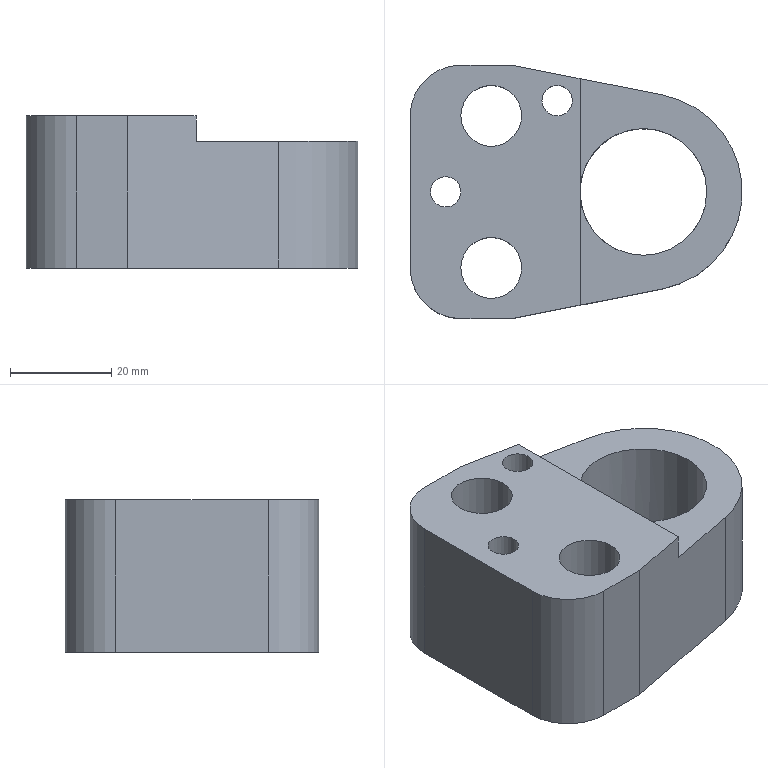Part | NX | features solid 2 | 1 solid | 25 faces | box 65.5 x 50 x 30 mm | volume 51666 mm3 | plane 13 | cylinder 12 | commonest cylinder face diameters 6 x2 8 x2 12 x2 17 x2 20 x2 25 x1
STEP:
#1=CARTESIAN_POINT('',(-1297.,441.948,99.));
#2=VERTEX_POINT('',#1);
#3=CARTESIAN_POINT('',(-1301.,441.948,99.));
#4=DIRECTION('',(0.,0.,-1.));
#5=DIRECTION('',(1.,0.,0.));
#6=AXIS2_PLACEMENT_3D('',#3,#4,#5);
#7=CIRCLE('',#6,4.);
#8=EDGE_CURVE('',#2,#2,#7,.F.);
#9=ORIENTED_EDGE('',*,*,#8,.T.);
#10=EDGE_LOOP('',(#9));
#11=FACE_BOUND('',#10,.T.);
#12=CARTESIAN_POINT('',(-1300.5,456.948,99.));
#13=VERTEX_POINT('',#12);
#14=CARTESIAN_POINT('',(-1292.,456.948,99.));
#15=DIRECTION('',(0.,0.,1.));
#16=DIRECTION('',(-1.,0.,0.));
#17=AXIS2_PLACEMENT_3D('',#14,#15,#16);
#18=CIRCLE('',#17,8.5);
#19=EDGE_CURVE('',#13,#13,#18,.T.);
#20=ORIENTED_EDGE('',*,*,#19,.T.);
#21=EDGE_LOOP('',(#20));
#22=FACE_BOUND('',#21,.T.);
#23=CARTESIAN_POINT('',(-1300.5,426.948,99.));
#24=VERTEX_POINT('',#23);
#25=CARTESIAN_POINT('',(-1292.,426.948,99.));
#26=DIRECTION('',(0.,0.,1.));
#27=DIRECTION('',(-1.,0.,0.));
#28=AXIS2_PLACEMENT_3D('',#25,#26,#27);
#29=CIRCLE('',#28,8.5);
#30=EDGE_CURVE('',#24,#24,#29,.T.);
#31=ORIENTED_EDGE('',*,*,#30,.T.);
#32=EDGE_LOOP('',(#31));
#33=FACE_BOUND('',#32,.T.);
#34=CARTESIAN_POINT('',(-1249.5,441.948,99.));
#35=VERTEX_POINT('',#34);
#36=CARTESIAN_POINT('',(-1262.,441.948,99.));
#37=DIRECTION('',(0.,0.,-1.));
#38=DIRECTION('',(1.,0.,0.));
#39=AXIS2_PLACEMENT_3D('',#36,#37,#38);
#40=CIRCLE('',#39,12.5);
#41=EDGE_CURVE('',#35,#35,#40,.T.);
#42=ORIENTED_EDGE('',*,*,#41,.F.);
#43=EDGE_LOOP('',(#42));
#44=FACE_BOUND('',#43,.T.);
#45=CARTESIAN_POINT('',(-1258.229,422.816,99.));
#46=VERTEX_POINT('',#45);
#47=CARTESIAN_POINT('',(-1288.,416.948,99.));
#48=VERTEX_POINT('',#47);
#49=CARTESIAN_POINT('',(-1258.229,422.816,99.));
#50=DIRECTION('',(-0.9811,-0.1934,0.));
#51=VECTOR('',#50,1000.);
#52=LINE('',#49,#51);
#53=EDGE_CURVE('',#46,#48,#52,.T.);
#54=ORIENTED_EDGE('',*,*,#53,.T.);
#55=CARTESIAN_POINT('',(-1298.,416.948,99.));
#56=VERTEX_POINT('',#55);
#57=CARTESIAN_POINT('',(-1288.,416.948,99.));
#58=DIRECTION('',(-1.,0.,0.));
#59=VECTOR('',#58,1000.);
#60=LINE('',#57,#59);
#61=EDGE_CURVE('',#48,#56,#60,.T.);
#62=ORIENTED_EDGE('',*,*,#61,.T.);
#63=CARTESIAN_POINT('',(-1308.,426.948,99.));
#64=VERTEX_POINT('',#63);
#65=CARTESIAN_POINT('',(-1298.,426.948,99.));
#66=DIRECTION('',(0.,0.,1.));
#67=DIRECTION('',(-1.,0.,0.));
#68=AXIS2_PLACEMENT_3D('',#65,#66,#67);
#69=CIRCLE('',#68,10.);
#70=EDGE_CURVE('',#64,#56,#69,.T.);
#71=ORIENTED_EDGE('',*,*,#70,.F.);
#72=CARTESIAN_POINT('',(-1308.,456.948,99.));
#73=VERTEX_POINT('',#72);
#74=CARTESIAN_POINT('',(-1308.,426.948,99.));
#75=DIRECTION('',(0.,1.,0.));
#76=VECTOR('',#75,1000.);
#77=LINE('',#74,#76);
#78=EDGE_CURVE('',#64,#73,#77,.T.);
#79=ORIENTED_EDGE('',*,*,#78,.T.);
#80=CARTESIAN_POINT('',(-1298.,466.948,99.));
#81=VERTEX_POINT('',#80);
#82=CARTESIAN_POINT('',(-1298.,456.948,99.));
#83=DIRECTION('',(0.,0.,1.));
#84=DIRECTION('',(-1.,0.,0.));
#85=AXIS2_PLACEMENT_3D('',#82,#83,#84);
#86=CIRCLE('',#85,10.);
#87=EDGE_CURVE('',#81,#73,#86,.T.);
#88=ORIENTED_EDGE('',*,*,#87,.F.);
#89=CARTESIAN_POINT('',(-1288.,466.948,99.));
#90=VERTEX_POINT('',#89);
#91=CARTESIAN_POINT('',(-1288.,466.948,99.));
#92=DIRECTION('',(-1.,0.,0.));
#93=VECTOR('',#92,1000.);
#94=LINE('',#91,#93);
#95=EDGE_CURVE('',#90,#81,#94,.T.);
#96=ORIENTED_EDGE('',*,*,#95,.F.);
#97=CARTESIAN_POINT('',(-1258.229,461.08,99.));
#98=VERTEX_POINT('',#97);
#99=CARTESIAN_POINT('',(-1258.229,461.08,99.));
#100=DIRECTION('',(-0.9811,0.1934,0.));
#101=VECTOR('',#100,1000.);
#102=LINE('',#99,#101);
#103=EDGE_CURVE('',#98,#90,#102,.T.);
#104=ORIENTED_EDGE('',*,*,#103,.F.);
#105=CARTESIAN_POINT('',(-1262.,441.948,99.));
#106=DIRECTION('',(0.,0.,1.));
#107=DIRECTION('',(-1.,0.,0.));
#108=AXIS2_PLACEMENT_3D('',#105,#106,#107);
#109=CIRCLE('',#108,19.5);
#110=EDGE_CURVE('',#46,#98,#109,.T.);
#111=ORIENTED_EDGE('',*,*,#110,.F.);
#112=EDGE_LOOP('',(#54,#62,#71,#79,#88,#96,#104,#111));
#113=FACE_BOUND('',#112,.T.);
#114=CARTESIAN_POINT('',(-1275.,459.948,99.));
#115=VERTEX_POINT('',#114);
#116=CARTESIAN_POINT('',(-1279.,459.948,99.));
#117=DIRECTION('',(0.,0.,-1.));
#118=DIRECTION('',(1.,0.,0.));
#119=AXIS2_PLACEMENT_3D('',#116,#117,#118);
#120=CIRCLE('',#119,4.);
#121=EDGE_CURVE('',#115,#115,#120,.F.);
#122=ORIENTED_EDGE('',*,*,#121,.T.);
#123=EDGE_LOOP('',(#122));
#124=FACE_BOUND('',#123,.T.);
#125=CARTESIAN_POINT('',(-1298.,426.948,99.));
#126=DIRECTION('',(0.,0.,-1.));
#127=DIRECTION('',(-1.,0.,0.));
#128=AXIS2_PLACEMENT_3D('',#125,#126,#127);
#129=PLANE('',#128);
#130=ADVANCED_FACE('',(#11,#22,#33,#44,#113,#124),#129,.T.);
#131=CARTESIAN_POINT('',(-1304.,441.948,129.));
#132=VERTEX_POINT('',#131);
#133=CARTESIAN_POINT('',(-1301.,441.948,129.));
#134=DIRECTION('',(0.,0.,1.));
#135=DIRECTION('',(-1.,0.,0.));
#136=AXIS2_PLACEMENT_3D('',#133,#134,#135);
#137=CIRCLE('',#136,3.);
#138=EDGE_CURVE('',#132,#132,#137,.T.);
#139=ORIENTED_EDGE('',*,*,#138,.T.);
#140=EDGE_LOOP('',(#139));
#141=FACE_BOUND('',#140,.T.);
#142=CARTESIAN_POINT('',(-1304.,441.948,119.));
#143=VERTEX_POINT('',#142);
#144=CARTESIAN_POINT('',(-1301.,441.948,119.));
#145=DIRECTION('',(0.,0.,1.));
#146=DIRECTION('',(-1.,0.,0.));
#147=AXIS2_PLACEMENT_3D('',#144,#145,#146);
#148=CIRCLE('',#147,3.);
#149=EDGE_CURVE('',#143,#143,#148,.T.);
#150=ORIENTED_EDGE('',*,*,#149,.F.);
#151=EDGE_LOOP('',(#150));
#152=FACE_BOUND('',#151,.T.);
#153=CARTESIAN_POINT('',(-1301.,441.948,99.));
#154=DIRECTION('',(0.,0.,1.));
#155=DIRECTION('',(1.,0.,0.));
#156=AXIS2_PLACEMENT_3D('',#153,#154,#155);
#157=CYLINDRICAL_SURFACE('',#156,3.);
#158=ADVANCED_FACE('',(#141,#152),#157,.F.);
#159=CARTESIAN_POINT('',(-1298.,456.948,129.));
#160=VERTEX_POINT('',#159);
#161=CARTESIAN_POINT('',(-1292.,456.948,129.));
#162=DIRECTION('',(0.,0.,1.));
#163=DIRECTION('',(-1.,0.,0.));
#164=AXIS2_PLACEMENT_3D('',#161,#162,#163);
#165=CIRCLE('',#164,6.);
#166=EDGE_CURVE('',#160,#160,#165,.T.);
#167=ORIENTED_EDGE('',*,*,#166,.T.);
#168=EDGE_LOOP('',(#167));
#169=FACE_BOUND('',#168,.T.);
#170=CARTESIAN_POINT('',(-1298.,456.948,111.));
#171=VERTEX_POINT('',#170);
#172=CARTESIAN_POINT('',(-1292.,456.948,111.));
#173=DIRECTION('',(0.,0.,1.));
#174=DIRECTION('',(-1.,0.,0.));
#175=AXIS2_PLACEMENT_3D('',#172,#173,#174);
#176=CIRCLE('',#175,6.);
#177=EDGE_CURVE('',#171,#171,#176,.T.);
#178=ORIENTED_EDGE('',*,*,#177,.F.);
#179=EDGE_LOOP('',(#178));
#180=FACE_BOUND('',#179,.T.);
#181=CARTESIAN_POINT('',(-1292.,456.948,99.));
#182=DIRECTION('',(0.,0.,1.));
#183=DIRECTION('',(1.,0.,0.));
#184=AXIS2_PLACEMENT_3D('',#181,#182,#183);
#185=CYLINDRICAL_SURFACE('',#184,6.);
#186=ADVANCED_FACE('',(#169,#180),#185,.F.);
#187=CARTESIAN_POINT('',(-1298.,426.948,129.));
#188=VERTEX_POINT('',#187);
#189=CARTESIAN_POINT('',(-1292.,426.948,129.));
#190=DIRECTION('',(0.,0.,1.));
#191=DIRECTION('',(-1.,0.,0.));
#192=AXIS2_PLACEMENT_3D('',#189,#190,#191);
#193=CIRCLE('',#192,6.);
#194=EDGE_CURVE('',#188,#188,#193,.T.);
#195=ORIENTED_EDGE('',*,*,#194,.T.);
#196=EDGE_LOOP('',(#195));
#197=FACE_BOUND('',#196,.T.);
#198=CARTESIAN_POINT('',(-1298.,426.948,111.));
#199=VERTEX_POINT('',#198);
#200=CARTESIAN_POINT('',(-1292.,426.948,111.));
#201=DIRECTION('',(0.,0.,1.));
#202=DIRECTION('',(-1.,0.,0.));
#203=AXIS2_PLACEMENT_3D('',#200,#201,#202);
#204=CIRCLE('',#203,6.);
#205=EDGE_CURVE('',#199,#199,#204,.T.);
#206=ORIENTED_EDGE('',*,*,#205,.F.);
#207=EDGE_LOOP('',(#206));
#208=FACE_BOUND('',#207,.T.);
#209=CARTESIAN_POINT('',(-1292.,426.948,99.));
#210=DIRECTION('',(0.,0.,1.));
#211=DIRECTION('',(1.,0.,0.));
#212=AXIS2_PLACEMENT_3D('',#209,#210,#211);
#213=CYLINDRICAL_SURFACE('',#212,6.);
#214=ADVANCED_FACE('',(#197,#208),#213,.F.);
#215=CARTESIAN_POINT('',(-1282.,459.948,129.));
#216=VERTEX_POINT('',#215);
#217=CARTESIAN_POINT('',(-1279.,459.948,129.));
#218=DIRECTION('',(0.,0.,1.));
#219=DIRECTION('',(-1.,0.,0.));
#220=AXIS2_PLACEMENT_3D('',#217,#218,#219);
#221=CIRCLE('',#220,3.);
#222=EDGE_CURVE('',#216,#216,#221,.T.);
#223=ORIENTED_EDGE('',*,*,#222,.F.);
#224=EDGE_LOOP('',(#223));
#225=FACE_BOUND('',#224,.T.);
#226=ORIENTED_EDGE('',*,*,#166,.F.);
#227=EDGE_LOOP('',(#226));
#228=FACE_BOUND('',#227,.T.);
#229=CARTESIAN_POINT('',(-1274.5,464.287,129.));
#230=VERTEX_POINT('',#229);
#231=CARTESIAN_POINT('',(-1288.,466.948,129.));
#232=VERTEX_POINT('',#231);
#233=CARTESIAN_POINT('',(-1258.229,461.08,129.));
#234=DIRECTION('',(-0.9811,0.1934,0.));
#235=VECTOR('',#234,1000.);
#236=LINE('',#233,#235);
#237=EDGE_CURVE('',#230,#232,#236,.T.);
#238=ORIENTED_EDGE('',*,*,#237,.T.);
#239=CARTESIAN_POINT('',(-1298.,466.948,129.));
#240=VERTEX_POINT('',#239);
#241=CARTESIAN_POINT('',(-1288.,466.948,129.));
#242=DIRECTION('',(-1.,0.,0.));
#243=VECTOR('',#242,1000.);
#244=LINE('',#241,#243);
#245=EDGE_CURVE('',#232,#240,#244,.T.);
#246=ORIENTED_EDGE('',*,*,#245,.T.);
#247=CARTESIAN_POINT('',(-1308.,456.948,129.));
#248=VERTEX_POINT('',#247);
#249=CARTESIAN_POINT('',(-1298.,456.948,129.));
#250=DIRECTION('',(0.,0.,1.));
#251=DIRECTION('',(-1.,0.,0.));
#252=AXIS2_PLACEMENT_3D('',#249,#250,#251);
#253=CIRCLE('',#252,10.);
#254=EDGE_CURVE('',#240,#248,#253,.T.);
#255=ORIENTED_EDGE('',*,*,#254,.T.);
#256=CARTESIAN_POINT('',(-1308.,426.948,129.));
#257=VERTEX_POINT('',#256);
#258=CARTESIAN_POINT('',(-1308.,426.948,129.));
#259=DIRECTION('',(0.,1.,0.));
#260=VECTOR('',#259,1000.);
#261=LINE('',#258,#260);
#262=EDGE_CURVE('',#257,#248,#261,.T.);
#263=ORIENTED_EDGE('',*,*,#262,.F.);
#264=CARTESIAN_POINT('',(-1298.,416.948,129.));
#265=VERTEX_POINT('',#264);
#266=CARTESIAN_POINT('',(-1298.,426.948,129.));
#267=DIRECTION('',(0.,0.,1.));
#268=DIRECTION('',(-1.,0.,0.));
#269=AXIS2_PLACEMENT_3D('',#266,#267,#268);
#270=CIRCLE('',#269,10.);
#271=EDGE_CURVE('',#257,#265,#270,.T.);
#272=ORIENTED_EDGE('',*,*,#271,.T.);
#273=CARTESIAN_POINT('',(-1288.,416.948,129.));
#274=VERTEX_POINT('',#273);
#275=CARTESIAN_POINT('',(-1288.,416.948,129.));
#276=DIRECTION('',(-1.,0.,0.));
#277=VECTOR('',#276,1000.);
#278=LINE('',#275,#277);
#279=EDGE_CURVE('',#274,#265,#278,.T.);
#280=ORIENTED_EDGE('',*,*,#279,.F.);
#281=CARTESIAN_POINT('',(-1274.5,419.609,129.));
#282=VERTEX_POINT('',#281);
#283=CARTESIAN_POINT('',(-1258.229,422.816,129.));
#284=DIRECTION('',(-0.9811,-0.1934,0.));
#285=VECTOR('',#284,1000.);
#286=LINE('',#283,#285);
#287=EDGE_CURVE('',#282,#274,#286,.T.);
#288=ORIENTED_EDGE('',*,*,#287,.F.);
#289=CARTESIAN_POINT('',(-1274.5,419.609,129.));
#290=DIRECTION('',(0.,1.,0.));
#291=VECTOR('',#290,1000.);
#292=LINE('',#289,#291);
#293=EDGE_CURVE('',#282,#230,#292,.T.);
#294=ORIENTED_EDGE('',*,*,#293,.T.);
#295=EDGE_LOOP('',(#238,#246,#255,#263,#272,#280,#288,#294));
#296=FACE_BOUND('',#295,.T.);
#297=ORIENTED_EDGE('',*,*,#194,.F.);
#298=EDGE_LOOP('',(#297));
#299=FACE_BOUND('',#298,.T.);
#300=ORIENTED_EDGE('',*,*,#138,.F.);
#301=EDGE_LOOP('',(#300));
#302=FACE_BOUND('',#301,.T.);
#303=CARTESIAN_POINT('',(-1298.,426.948,129.));
#304=DIRECTION('',(0.,0.,-1.));
#305=DIRECTION('',(-1.,0.,0.));
#306=AXIS2_PLACEMENT_3D('',#303,#304,#305);
#307=PLANE('',#306);
#308=ADVANCED_FACE('',(#225,#228,#296,#299,#302),#307,.F.);
#309=CARTESIAN_POINT('',(-1274.5,419.609,124.));
#310=VERTEX_POINT('',#309);
#311=CARTESIAN_POINT('',(-1274.5,419.609,124.));
#312=DIRECTION('',(0.,0.,1.));
#313=VECTOR('',#312,1000.);
#314=LINE('',#311,#313);
#315=EDGE_CURVE('',#310,#282,#314,.T.);
#316=ORIENTED_EDGE('',*,*,#315,.T.);
#317=ORIENTED_EDGE('',*,*,#287,.T.);
#318=CARTESIAN_POINT('',(-1288.,416.948,99.));
#319=DIRECTION('',(0.,0.,1.));
#320=VECTOR('',#319,1000.);
#321=LINE('',#318,#320);
#322=EDGE_CURVE('',#48,#274,#321,.T.);
#323=ORIENTED_EDGE('',*,*,#322,.F.);
#324=ORIENTED_EDGE('',*,*,#53,.F.);
#325=CARTESIAN_POINT('',(-1258.229,422.816,124.));
#326=VERTEX_POINT('',#325);
#327=CARTESIAN_POINT('',(-1258.229,422.816,99.));
#328=DIRECTION('',(0.,0.,1.));
#329=VECTOR('',#328,1000.);
#330=LINE('',#327,#329);
#331=EDGE_CURVE('',#46,#326,#330,.T.);
#332=ORIENTED_EDGE('',*,*,#331,.T.);
#333=CARTESIAN_POINT('',(-1274.5,419.609,124.));
#334=DIRECTION('',(0.9811,0.1934,0.));
#335=VECTOR('',#334,1000.);
#336=LINE('',#333,#335);
#337=EDGE_CURVE('',#310,#326,#336,.T.);
#338=ORIENTED_EDGE('',*,*,#337,.F.);
#339=EDGE_LOOP('',(#316,#317,#323,#324,#332,#338));
#340=FACE_BOUND('',#339,.T.);
#341=CARTESIAN_POINT('',(-1258.229,422.816,99.));
#342=DIRECTION('',(0.1934,-0.9811,0.));
#343=DIRECTION('',(-0.9811,-0.1934,0.));
#344=AXIS2_PLACEMENT_3D('',#341,#342,#343);
#345=PLANE('',#344);
#346=ADVANCED_FACE('',(#340),#345,.T.);
#347=ORIENTED_EDGE('',*,*,#279,.T.);
#348=CARTESIAN_POINT('',(-1298.,416.948,99.));
#349=DIRECTION('',(0.,0.,1.));
#350=VECTOR('',#349,1000.);
#351=LINE('',#348,#350);
#352=EDGE_CURVE('',#56,#265,#351,.T.);
#353=ORIENTED_EDGE('',*,*,#352,.F.);
#354=ORIENTED_EDGE('',*,*,#61,.F.);
#355=ORIENTED_EDGE('',*,*,#322,.T.);
#356=EDGE_LOOP('',(#347,#353,#354,#355));
#357=FACE_BOUND('',#356,.T.);
#358=CARTESIAN_POINT('',(-1288.,416.948,99.));
#359=DIRECTION('',(0.,-1.,0.));
#360=DIRECTION('',(-1.,0.,0.));
#361=AXIS2_PLACEMENT_3D('',#358,#359,#360);
#362=PLANE('',#361);
#363=ADVANCED_FACE('',(#357),#362,.T.);
#364=ORIENTED_EDGE('',*,*,#271,.F.);
#365=CARTESIAN_POINT('',(-1308.,426.948,99.));
#366=DIRECTION('',(0.,0.,1.));
#367=VECTOR('',#366,1000.);
#368=LINE('',#365,#367);
#369=EDGE_CURVE('',#64,#257,#368,.T.);
#370=ORIENTED_EDGE('',*,*,#369,.F.);
#371=ORIENTED_EDGE('',*,*,#70,.T.);
#372=ORIENTED_EDGE('',*,*,#352,.T.);
#373=EDGE_LOOP('',(#364,#370,#371,#372));
#374=FACE_BOUND('',#373,.T.);
#375=CARTESIAN_POINT('',(-1298.,426.948,99.));
#376=DIRECTION('',(0.,0.,1.));
#377=DIRECTION('',(1.,0.,0.));
#378=AXIS2_PLACEMENT_3D('',#375,#376,#377);
#379=CYLINDRICAL_SURFACE('',#378,10.);
#380=ADVANCED_FACE('',(#374),#379,.T.);
#381=ORIENTED_EDGE('',*,*,#262,.T.);
#382=CARTESIAN_POINT('',(-1308.,456.948,99.));
#383=DIRECTION('',(0.,0.,1.));
#384=VECTOR('',#383,1000.);
#385=LINE('',#382,#384);
#386=EDGE_CURVE('',#73,#248,#385,.T.);
#387=ORIENTED_EDGE('',*,*,#386,.F.);
#388=ORIENTED_EDGE('',*,*,#78,.F.);
#389=ORIENTED_EDGE('',*,*,#369,.T.);
#390=EDGE_LOOP('',(#381,#387,#388,#389));
#391=FACE_BOUND('',#390,.T.);
#392=CARTESIAN_POINT('',(-1308.,426.948,99.));
#393=DIRECTION('',(-1.,0.,0.));
#394=DIRECTION('',(0.,0.,1.));
#395=AXIS2_PLACEMENT_3D('',#392,#393,#394);
#396=PLANE('',#395);
#397=ADVANCED_FACE('',(#391),#396,.T.);
#398=ORIENTED_EDGE('',*,*,#254,.F.);
#399=CARTESIAN_POINT('',(-1298.,466.948,99.));
#400=DIRECTION('',(0.,0.,1.));
#401=VECTOR('',#400,1000.);
#402=LINE('',#399,#401);
#403=EDGE_CURVE('',#81,#240,#402,.T.);
#404=ORIENTED_EDGE('',*,*,#403,.F.);
#405=ORIENTED_EDGE('',*,*,#87,.T.);
#406=ORIENTED_EDGE('',*,*,#386,.T.);
#407=EDGE_LOOP('',(#398,#404,#405,#406));
#408=FACE_BOUND('',#407,.T.);
#409=CARTESIAN_POINT('',(-1298.,456.948,99.));
#410=DIRECTION('',(0.,0.,1.));
#411=DIRECTION('',(1.,0.,0.));
#412=AXIS2_PLACEMENT_3D('',#409,#410,#411);
#413=CYLINDRICAL_SURFACE('',#412,10.);
#414=ADVANCED_FACE('',(#408),#413,.T.);
#415=ORIENTED_EDGE('',*,*,#245,.F.);
#416=CARTESIAN_POINT('',(-1288.,466.948,99.));
#417=DIRECTION('',(0.,0.,1.));
#418=VECTOR('',#417,1000.);
#419=LINE('',#416,#418);
#420=EDGE_CURVE('',#90,#232,#419,.T.);
#421=ORIENTED_EDGE('',*,*,#420,.F.);
#422=ORIENTED_EDGE('',*,*,#95,.T.);
#423=ORIENTED_EDGE('',*,*,#403,.T.);
#424=EDGE_LOOP('',(#415,#421,#422,#423));
#425=FACE_BOUND('',#424,.T.);
#426=CARTESIAN_POINT('',(-1288.,466.948,99.));
#427=DIRECTION('',(0.,-1.,0.));
#428=DIRECTION('',(0.,0.,1.));
#429=AXIS2_PLACEMENT_3D('',#426,#427,#428);
#430=PLANE('',#429);
#431=ADVANCED_FACE('',(#425),#430,.F.);
#432=CARTESIAN_POINT('',(-1274.5,464.287,124.));
#433=VERTEX_POINT('',#432);
#434=CARTESIAN_POINT('',(-1258.229,461.08,124.));
#435=VERTEX_POINT('',#434);
#436=CARTESIAN_POINT('',(-1274.5,464.287,124.));
#437=DIRECTION('',(0.9811,-0.1934,0.));
#438=VECTOR('',#437,1000.);
#439=LINE('',#436,#438);
#440=EDGE_CURVE('',#433,#435,#439,.T.);
#441=ORIENTED_EDGE('',*,*,#440,.T.);
#442=CARTESIAN_POINT('',(-1258.229,461.08,99.));
#443=DIRECTION('',(0.,0.,1.));
#444=VECTOR('',#443,1000.);
#445=LINE('',#442,#444);
#446=EDGE_CURVE('',#98,#435,#445,.T.);
#447=ORIENTED_EDGE('',*,*,#446,.F.);
#448=ORIENTED_EDGE('',*,*,#103,.T.);
#449=ORIENTED_EDGE('',*,*,#420,.T.);
#450=ORIENTED_EDGE('',*,*,#237,.F.);
#451=CARTESIAN_POINT('',(-1274.5,464.287,124.));
#452=DIRECTION('',(0.,0.,1.));
#453=VECTOR('',#452,1000.);
#454=LINE('',#451,#453);
#455=EDGE_CURVE('',#433,#230,#454,.T.);
#456=ORIENTED_EDGE('',*,*,#455,.F.);
#457=EDGE_LOOP('',(#441,#447,#448,#449,#450,#456));
#458=FACE_BOUND('',#457,.T.);
#459=CARTESIAN_POINT('',(-1258.229,461.08,99.));
#460=DIRECTION('',(-0.1934,-0.9811,0.));
#461=DIRECTION('',(-0.9811,0.1934,0.));
#462=AXIS2_PLACEMENT_3D('',#459,#460,#461);
#463=PLANE('',#462);
#464=ADVANCED_FACE('',(#458),#463,.F.);
#465=ORIENTED_EDGE('',*,*,#331,.F.);
#466=ORIENTED_EDGE('',*,*,#110,.T.);
#467=ORIENTED_EDGE('',*,*,#446,.T.);
#468=CARTESIAN_POINT('',(-1262.,441.948,124.));
#469=DIRECTION('',(0.,0.,1.));
#470=DIRECTION('',(-1.,0.,0.));
#471=AXIS2_PLACEMENT_3D('',#468,#469,#470);
#472=CIRCLE('',#471,19.5);
#473=EDGE_CURVE('',#326,#435,#472,.T.);
#474=ORIENTED_EDGE('',*,*,#473,.F.);
#475=EDGE_LOOP('',(#465,#466,#467,#474));
#476=FACE_BOUND('',#475,.T.);
#477=CARTESIAN_POINT('',(-1262.,441.948,99.));
#478=DIRECTION('',(0.,0.,1.));
#479=DIRECTION('',(1.,0.,0.));
#480=AXIS2_PLACEMENT_3D('',#477,#478,#479);
#481=CYLINDRICAL_SURFACE('',#480,19.5);
#482=ADVANCED_FACE('',(#476),#481,.T.);
#483=CARTESIAN_POINT('',(-1274.5,441.948,124.));
#484=VERTEX_POINT('',#483);
#485=CARTESIAN_POINT('',(-1262.,441.948,124.));
#486=DIRECTION('',(0.,0.,1.));
#487=DIRECTION('',(-1.,0.,0.));
#488=AXIS2_PLACEMENT_3D('',#485,#486,#487);
#489=CIRCLE('',#488,12.5);
#490=EDGE_CURVE('',#484,#484,#489,.F.);
#491=ORIENTED_EDGE('',*,*,#490,.F.);
#492=EDGE_LOOP('',(#491));
#493=FACE_BOUND('',#492,.T.);
#494=ORIENTED_EDGE('',*,*,#41,.T.);
#495=EDGE_LOOP('',(#494));
#496=FACE_BOUND('',#495,.T.);
#497=CARTESIAN_POINT('',(-1262.,441.948,99.));
#498=DIRECTION('',(0.,0.,1.));
#499=DIRECTION('',(1.,0.,0.));
#500=AXIS2_PLACEMENT_3D('',#497,#498,#499);
#501=CYLINDRICAL_SURFACE('',#500,12.5);
#502=ADVANCED_FACE('',(#493,#496),#501,.F.);
#503=ORIENTED_EDGE('',*,*,#293,.F.);
#504=ORIENTED_EDGE('',*,*,#315,.F.);
#505=CARTESIAN_POINT('',(-1274.5,419.609,124.));
#506=DIRECTION('',(0.,1.,0.));
#507=VECTOR('',#506,1000.);
#508=LINE('',#505,#507);
#509=EDGE_CURVE('',#310,#484,#508,.T.);
#510=ORIENTED_EDGE('',*,*,#509,.T.);
#511=CARTESIAN_POINT('',(-1274.5,419.609,124.));
#512=DIRECTION('',(0.,1.,0.));
#513=VECTOR('',#512,1000.);
#514=LINE('',#511,#513);
#515=EDGE_CURVE('',#484,#433,#514,.T.);
#516=ORIENTED_EDGE('',*,*,#515,.T.);
#517=ORIENTED_EDGE('',*,*,#455,.T.);
#518=EDGE_LOOP('',(#503,#504,#510,#516,#517));
#519=FACE_BOUND('',#518,.T.);
#520=CARTESIAN_POINT('',(-1274.5,419.609,124.));
#521=DIRECTION('',(-1.,0.,0.));
#522=DIRECTION('',(0.,1.,0.));
#523=AXIS2_PLACEMENT_3D('',#520,#521,#522);
#524=PLANE('',#523);
#525=ADVANCED_FACE('',(#519),#524,.F.);
#526=ORIENTED_EDGE('',*,*,#515,.F.);
#527=ORIENTED_EDGE('',*,*,#490,.T.);
#528=ORIENTED_EDGE('',*,*,#509,.F.);
#529=ORIENTED_EDGE('',*,*,#337,.T.);
#530=ORIENTED_EDGE('',*,*,#473,.T.);
#531=ORIENTED_EDGE('',*,*,#440,.F.);
#532=EDGE_LOOP('',(#526,#527,#528,#529,#530,#531));
#533=FACE_BOUND('',#532,.T.);
#534=CARTESIAN_POINT('',(-1262.,441.948,124.));
#535=DIRECTION('',(0.,0.,-1.));
#536=DIRECTION('',(-1.,0.,0.));
#537=AXIS2_PLACEMENT_3D('',#534,#535,#536);
#538=PLANE('',#537);
#539=ADVANCED_FACE('',(#533),#538,.F.);
#540=CARTESIAN_POINT('',(-1282.,459.948,119.));
#541=VERTEX_POINT('',#540);
#542=CARTESIAN_POINT('',(-1279.,459.948,119.));
#543=DIRECTION('',(0.,0.,1.));
#544=DIRECTION('',(-1.,0.,0.));
#545=AXIS2_PLACEMENT_3D('',#542,#543,#544);
#546=CIRCLE('',#545,3.);
#547=EDGE_CURVE('',#541,#541,#546,.T.);
#548=ORIENTED_EDGE('',*,*,#547,.F.);
#549=EDGE_LOOP('',(#548));
#550=FACE_BOUND('',#549,.T.);
#551=ORIENTED_EDGE('',*,*,#222,.T.);
#552=EDGE_LOOP('',(#551));
#553=FACE_BOUND('',#552,.T.);
#554=CARTESIAN_POINT('',(-1279.,459.948,99.));
#555=DIRECTION('',(0.,0.,1.));
#556=DIRECTION('',(1.,0.,0.));
#557=AXIS2_PLACEMENT_3D('',#554,#555,#556);
#558=CYLINDRICAL_SURFACE('',#557,3.);
#559=ADVANCED_FACE('',(#550,#553),#558,.F.);
#560=CARTESIAN_POINT('',(-1300.5,426.948,111.));
#561=VERTEX_POINT('',#560);
#562=CARTESIAN_POINT('',(-1292.,426.948,111.));
#563=DIRECTION('',(0.,0.,1.));
#564=DIRECTION('',(-1.,0.,0.));
#565=AXIS2_PLACEMENT_3D('',#562,#563,#564);
#566=CIRCLE('',#565,8.5);
#567=EDGE_CURVE('',#561,#561,#566,.T.);
#568=ORIENTED_EDGE('',*,*,#567,.T.);
#569=EDGE_LOOP('',(#568));
#570=FACE_BOUND('',#569,.T.);
#571=ORIENTED_EDGE('',*,*,#30,.F.);
#572=EDGE_LOOP('',(#571));
#573=FACE_BOUND('',#572,.T.);
#574=CARTESIAN_POINT('',(-1292.,426.948,111.));
#575=DIRECTION('',(0.,0.,-1.));
#576=DIRECTION('',(-1.,0.,0.));
#577=AXIS2_PLACEMENT_3D('',#574,#575,#576);
#578=CYLINDRICAL_SURFACE('',#577,8.5);
#579=ADVANCED_FACE('',(#570,#573),#578,.F.);
#580=ORIENTED_EDGE('',*,*,#205,.T.);
#581=EDGE_LOOP('',(#580));
#582=FACE_BOUND('',#581,.T.);
#583=ORIENTED_EDGE('',*,*,#567,.F.);
#584=EDGE_LOOP('',(#583));
#585=FACE_BOUND('',#584,.T.);
#586=CARTESIAN_POINT('',(-1292.,426.948,111.));
#587=DIRECTION('',(0.,0.,-1.));
#588=DIRECTION('',(-1.,0.,0.));
#589=AXIS2_PLACEMENT_3D('',#586,#587,#588);
#590=PLANE('',#589);
#591=ADVANCED_FACE('',(#582,#585),#590,.T.);
#592=CARTESIAN_POINT('',(-1300.5,456.948,111.));
#593=VERTEX_POINT('',#592);
#594=CARTESIAN_POINT('',(-1292.,456.948,111.));
#595=DIRECTION('',(0.,0.,1.));
#596=DIRECTION('',(-1.,0.,0.));
#597=AXIS2_PLACEMENT_3D('',#594,#595,#596);
#598=CIRCLE('',#597,8.5);
#599=EDGE_CURVE('',#593,#593,#598,.T.);
#600=ORIENTED_EDGE('',*,*,#599,.T.);
#601=EDGE_LOOP('',(#600));
#602=FACE_BOUND('',#601,.T.);
#603=ORIENTED_EDGE('',*,*,#19,.F.);
#604=EDGE_LOOP('',(#603));
#605=FACE_BOUND('',#604,.T.);
#606=CARTESIAN_POINT('',(-1292.,456.948,111.));
#607=DIRECTION('',(0.,0.,-1.));
#608=DIRECTION('',(-1.,0.,0.));
#609=AXIS2_PLACEMENT_3D('',#606,#607,#608);
#610=CYLINDRICAL_SURFACE('',#609,8.5);
#611=ADVANCED_FACE('',(#602,#605),#610,.F.);
#612=ORIENTED_EDGE('',*,*,#177,.T.);
#613=EDGE_LOOP('',(#612));
#614=FACE_BOUND('',#613,.T.);
#615=ORIENTED_EDGE('',*,*,#599,.F.);
#616=EDGE_LOOP('',(#615));
#617=FACE_BOUND('',#616,.T.);
#618=CARTESIAN_POINT('',(-1292.,456.948,111.));
#619=DIRECTION('',(0.,0.,-1.));
#620=DIRECTION('',(-1.,0.,0.));
#621=AXIS2_PLACEMENT_3D('',#618,#619,#620);
#622=PLANE('',#621);
#623=ADVANCED_FACE('',(#614,#617),#622,.T.);
#624=ORIENTED_EDGE('',*,*,#149,.T.);
#625=EDGE_LOOP('',(#624));
#626=FACE_BOUND('',#625,.T.);
#627=CARTESIAN_POINT('',(-1297.,441.948,119.));
#628=VERTEX_POINT('',#627);
#629=CARTESIAN_POINT('',(-1301.,441.948,119.));
#630=DIRECTION('',(0.,0.,-1.));
#631=DIRECTION('',(1.,0.,0.));
#632=AXIS2_PLACEMENT_3D('',#629,#630,#631);
#633=CIRCLE('',#632,4.);
#634=EDGE_CURVE('',#628,#628,#633,.F.);
#635=ORIENTED_EDGE('',*,*,#634,.F.);
#636=EDGE_LOOP('',(#635));
#637=FACE_BOUND('',#636,.T.);
#638=CARTESIAN_POINT('',(-1301.,441.948,119.));
#639=DIRECTION('',(0.,0.,1.));
#640=DIRECTION('',(1.,0.,0.));
#641=AXIS2_PLACEMENT_3D('',#638,#639,#640);
#642=PLANE('',#641);
#643=ADVANCED_FACE('',(#626,#637),#642,.F.);
#644=ORIENTED_EDGE('',*,*,#634,.T.);
#645=EDGE_LOOP('',(#644));
#646=FACE_BOUND('',#645,.T.);
#647=ORIENTED_EDGE('',*,*,#8,.F.);
#648=EDGE_LOOP('',(#647));
#649=FACE_BOUND('',#648,.T.);
#650=CARTESIAN_POINT('',(-1301.,441.948,99.));
#651=DIRECTION('',(0.,0.,1.));
#652=DIRECTION('',(1.,0.,0.));
#653=AXIS2_PLACEMENT_3D('',#650,#651,#652);
#654=CYLINDRICAL_SURFACE('',#653,4.);
#655=ADVANCED_FACE('',(#646,#649),#654,.F.);
#656=ORIENTED_EDGE('',*,*,#547,.T.);
#657=EDGE_LOOP('',(#656));
#658=FACE_BOUND('',#657,.T.);
#659=CARTESIAN_POINT('',(-1275.,459.948,119.));
#660=VERTEX_POINT('',#659);
#661=CARTESIAN_POINT('',(-1279.,459.948,119.));
#662=DIRECTION('',(0.,0.,-1.));
#663=DIRECTION('',(1.,0.,0.));
#664=AXIS2_PLACEMENT_3D('',#661,#662,#663);
#665=CIRCLE('',#664,4.);
#666=EDGE_CURVE('',#660,#660,#665,.F.);
#667=ORIENTED_EDGE('',*,*,#666,.F.);
#668=EDGE_LOOP('',(#667));
#669=FACE_BOUND('',#668,.T.);
#670=CARTESIAN_POINT('',(-1279.,459.948,119.));
#671=DIRECTION('',(0.,0.,1.));
#672=DIRECTION('',(1.,0.,0.));
#673=AXIS2_PLACEMENT_3D('',#670,#671,#672);
#674=PLANE('',#673);
#675=ADVANCED_FACE('',(#658,#669),#674,.F.);
#676=ORIENTED_EDGE('',*,*,#666,.T.);
#677=EDGE_LOOP('',(#676));
#678=FACE_BOUND('',#677,.T.);
#679=ORIENTED_EDGE('',*,*,#121,.F.);
#680=EDGE_LOOP('',(#679));
#681=FACE_BOUND('',#680,.T.);
#682=CARTESIAN_POINT('',(-1279.,459.948,99.));
#683=DIRECTION('',(0.,0.,1.));
#684=DIRECTION('',(1.,0.,0.));
#685=AXIS2_PLACEMENT_3D('',#682,#683,#684);
#686=CYLINDRICAL_SURFACE('',#685,4.);
#687=ADVANCED_FACE('',(#678,#681),#686,.F.);
#688=CLOSED_SHELL('',(#130,#158,#186,#214,#308,#346,#363,#380,#397,#414,#431,#464,#482,#502,#525,#539,#559,#579,#591,#611,#623,#643,#655,#675,#687));
#689=MANIFOLD_SOLID_BREP('',#688);
#690=(LENGTH_UNIT()NAMED_UNIT(*)SI_UNIT(.MILLI.,.METRE.));
#691=UNCERTAINTY_MEASURE_WITH_UNIT(LENGTH_MEASURE(0.00001),#690,'','');
#692=(NAMED_UNIT(*)PLANE_ANGLE_UNIT()SI_UNIT($,.RADIAN.));
#693=(NAMED_UNIT(*)SI_UNIT($,.STERADIAN.)SOLID_ANGLE_UNIT());
#694=(GEOMETRIC_REPRESENTATION_CONTEXT(3)GLOBAL_UNCERTAINTY_ASSIGNED_CONTEXT((#691))GLOBAL_UNIT_ASSIGNED_CONTEXT((#690,#692,#693))REPRESENTATION_CONTEXT('',''));
#695=ADVANCED_BREP_SHAPE_REPRESENTATION('',(#689),#694);